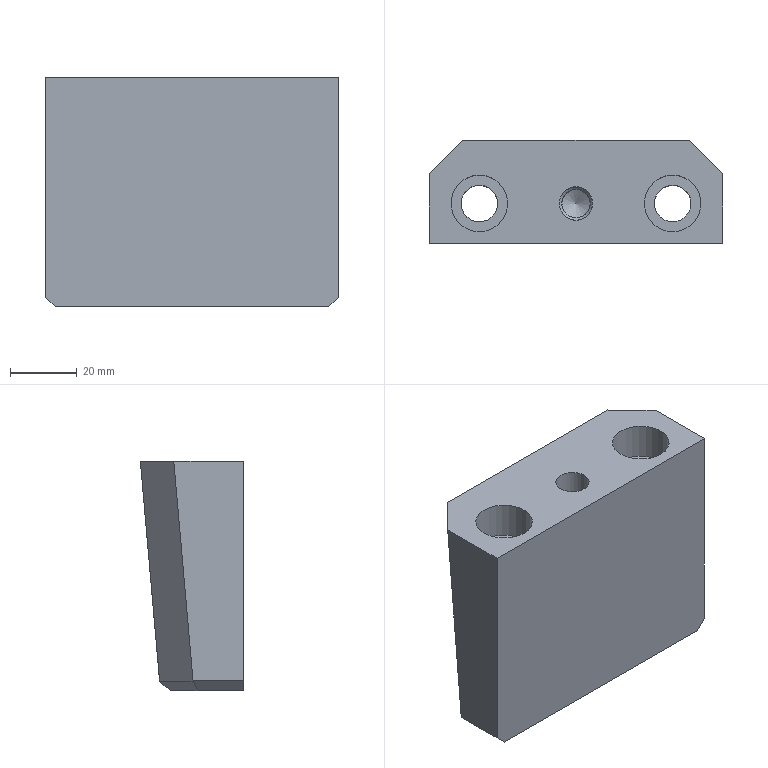Part | STEP file | P011002NM08-000 | 1 solid | 30 faces | box 88 x 31 x 69 mm | volume 144711 mm3 | plane 19 | cylinder 7 | cone 4 | commonest cylinder face diameters 11 x2 17 x2 8.5 x1 9.967 x1 10 x1